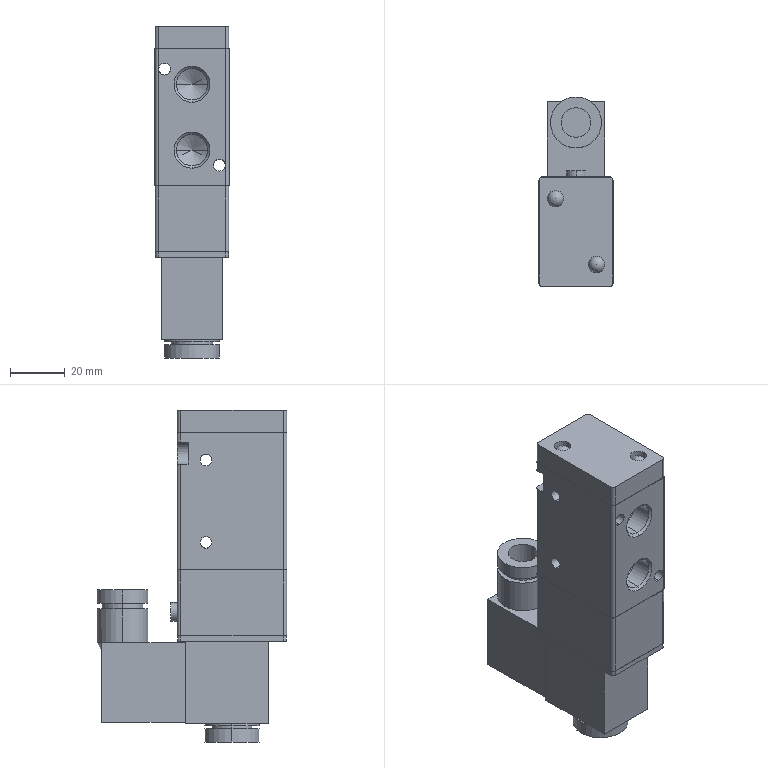Part | SolidWorks | 1 solid | 114 faces | box 27 x 69.2 x 120.9 mm | volume 129313 mm3 | cylinder 54 | plane 45 | cone 13 | sphere 2 | commonest cylinder face diameters 2.4 x18 4.3 x8 11.445 x6 6 x4 15 x4 18.6 x4